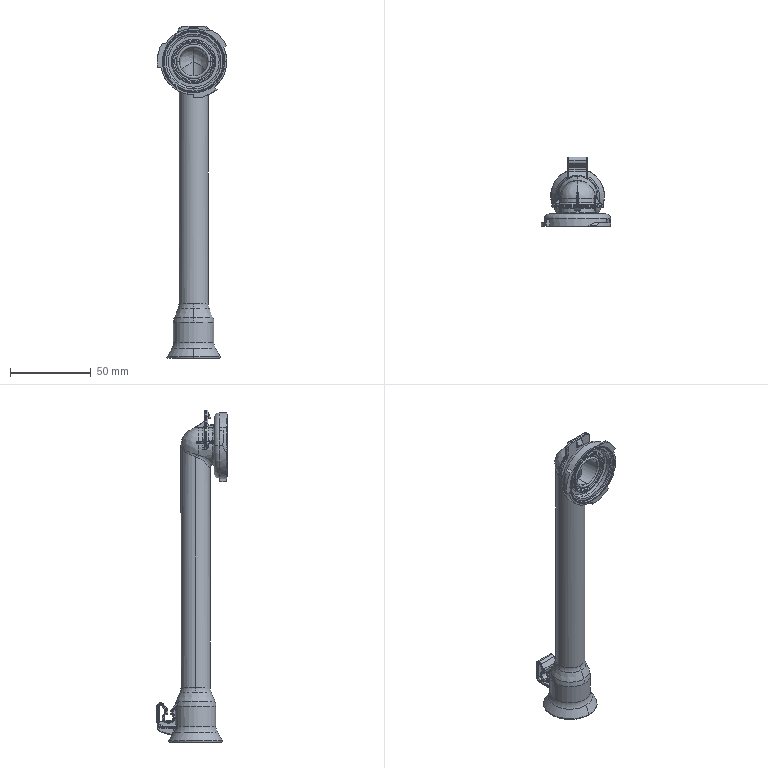Part | STEP file | MSBR-25 | 1 solid | 540 faces | box 43 x 43.4 x 205.2 mm | volume 28155 mm3 | cylinder 187 | torus 134 | spline 113 | plane 96 | cone 8 | sphere 2 | commonest cylinder face diameters 1 x70 0.6 x22 0.4 x16 2 x12 6 x9 1.4 x6